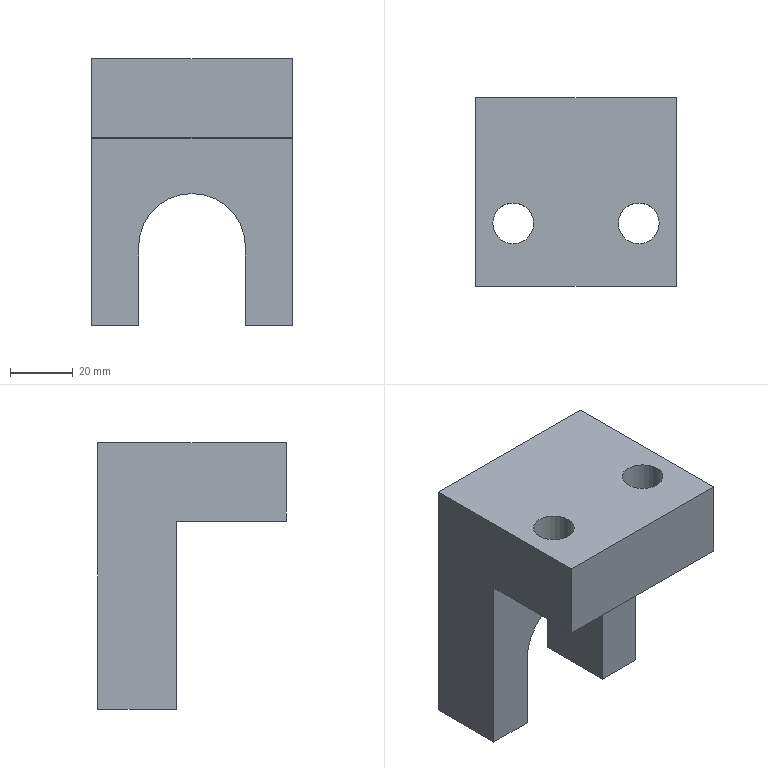Part | NX | features solid 2 | 1 solid | 19 faces | box 64 x 60 x 85 mm | volume 147325 mm3 | plane 13 | cylinder 6 | commonest cylinder face diameters 13 x2 20 x2 1 x1 34 x1
STEP:
#1=CARTESIAN_POINT('',(-138.,919.,-335.));
#2=VERTEX_POINT('',#1);
#3=CARTESIAN_POINT('',(-138.,919.,-310.));
#4=VERTEX_POINT('',#3);
#5=CARTESIAN_POINT('',(-138.,919.,-335.));
#6=DIRECTION('',(0.,0.,1.));
#7=VECTOR('',#6,1000.);
#8=LINE('',#5,#7);
#9=EDGE_CURVE('',#2,#4,#8,.T.);
#10=ORIENTED_EDGE('',*,*,#9,.T.);
#11=CARTESIAN_POINT('',(-202.,919.,-310.));
#12=VERTEX_POINT('',#11);
#13=CARTESIAN_POINT('',(-202.,919.,-310.));
#14=DIRECTION('',(-1.,0.,0.));
#15=VECTOR('',#14,1000.);
#16=LINE('',#13,#15);
#17=EDGE_CURVE('',#4,#12,#16,.T.);
#18=ORIENTED_EDGE('',*,*,#17,.T.);
#19=CARTESIAN_POINT('',(-202.,919.,-335.));
#20=VERTEX_POINT('',#19);
#21=CARTESIAN_POINT('',(-202.,919.,-335.));
#22=DIRECTION('',(0.,0.,-1.));
#23=VECTOR('',#22,1000.);
#24=LINE('',#21,#23);
#25=EDGE_CURVE('',#12,#20,#24,.T.);
#26=ORIENTED_EDGE('',*,*,#25,.T.);
#27=CARTESIAN_POINT('',(-202.,919.,-335.));
#28=DIRECTION('',(1.,0.,0.));
#29=VECTOR('',#28,1000.);
#30=LINE('',#27,#29);
#31=EDGE_CURVE('',#20,#2,#30,.T.);
#32=ORIENTED_EDGE('',*,*,#31,.T.);
#33=EDGE_LOOP('',(#10,#18,#26,#32));
#34=FACE_BOUND('',#33,.T.);
#35=CARTESIAN_POINT('',(-202.,919.,-335.));
#36=DIRECTION('',(0.,1.,0.));
#37=DIRECTION('',(-1.,0.,0.));
#38=AXIS2_PLACEMENT_3D('',#35,#36,#37);
#39=PLANE('',#38);
#40=ADVANCED_FACE('',(#34),#39,.F.);
#41=CARTESIAN_POINT('',(-153.,979.,-395.));
#42=VERTEX_POINT('',#41);
#43=CARTESIAN_POINT('',(-153.,954.,-395.));
#44=VERTEX_POINT('',#43);
#45=CARTESIAN_POINT('',(-153.,979.,-395.));
#46=DIRECTION('',(0.,-1.,0.));
#47=VECTOR('',#46,1000.);
#48=LINE('',#45,#47);
#49=EDGE_CURVE('',#42,#44,#48,.T.);
#50=ORIENTED_EDGE('',*,*,#49,.F.);
#51=CARTESIAN_POINT('',(-138.,979.,-395.));
#52=VERTEX_POINT('',#51);
#53=CARTESIAN_POINT('',(-138.,979.,-395.));
#54=DIRECTION('',(1.,0.,0.));
#55=VECTOR('',#54,1000.);
#56=LINE('',#53,#55);
#57=EDGE_CURVE('',#42,#52,#56,.T.);
#58=ORIENTED_EDGE('',*,*,#57,.T.);
#59=CARTESIAN_POINT('',(-138.,954.,-395.));
#60=VERTEX_POINT('',#59);
#61=CARTESIAN_POINT('',(-138.,979.,-395.));
#62=DIRECTION('',(0.,-1.,0.));
#63=VECTOR('',#62,1000.);
#64=LINE('',#61,#63);
#65=EDGE_CURVE('',#52,#60,#64,.T.);
#66=ORIENTED_EDGE('',*,*,#65,.T.);
#67=CARTESIAN_POINT('',(-138.,954.,-395.));
#68=DIRECTION('',(1.,0.,0.));
#69=VECTOR('',#68,1000.);
#70=LINE('',#67,#69);
#71=EDGE_CURVE('',#44,#60,#70,.T.);
#72=ORIENTED_EDGE('',*,*,#71,.F.);
#73=EDGE_LOOP('',(#50,#58,#66,#72));
#74=FACE_BOUND('',#73,.T.);
#75=CARTESIAN_POINT('',(-138.,979.,-395.));
#76=DIRECTION('',(0.,0.,1.));
#77=DIRECTION('',(0.,1.,0.));
#78=AXIS2_PLACEMENT_3D('',#75,#76,#77);
#79=PLANE('',#78);
#80=ADVANCED_FACE('',(#74),#79,.F.);
#81=CARTESIAN_POINT('',(-187.,954.,-395.));
#82=VERTEX_POINT('',#81);
#83=CARTESIAN_POINT('',(-187.,979.,-395.));
#84=VERTEX_POINT('',#83);
#85=CARTESIAN_POINT('',(-187.,979.,-395.));
#86=DIRECTION('',(0.,1.,0.));
#87=VECTOR('',#86,1000.);
#88=LINE('',#85,#87);
#89=EDGE_CURVE('',#82,#84,#88,.T.);
#90=ORIENTED_EDGE('',*,*,#89,.F.);
#91=CARTESIAN_POINT('',(-202.,954.,-395.));
#92=VERTEX_POINT('',#91);
#93=CARTESIAN_POINT('',(-138.,954.,-395.));
#94=DIRECTION('',(1.,0.,0.));
#95=VECTOR('',#94,1000.);
#96=LINE('',#93,#95);
#97=EDGE_CURVE('',#92,#82,#96,.T.);
#98=ORIENTED_EDGE('',*,*,#97,.F.);
#99=CARTESIAN_POINT('',(-202.,979.,-395.));
#100=VERTEX_POINT('',#99);
#101=CARTESIAN_POINT('',(-202.,979.,-395.));
#102=DIRECTION('',(0.,1.,0.));
#103=VECTOR('',#102,1000.);
#104=LINE('',#101,#103);
#105=EDGE_CURVE('',#92,#100,#104,.T.);
#106=ORIENTED_EDGE('',*,*,#105,.T.);
#107=CARTESIAN_POINT('',(-138.,979.,-395.));
#108=DIRECTION('',(1.,0.,0.));
#109=VECTOR('',#108,1000.);
#110=LINE('',#107,#109);
#111=EDGE_CURVE('',#100,#84,#110,.T.);
#112=ORIENTED_EDGE('',*,*,#111,.T.);
#113=EDGE_LOOP('',(#90,#98,#106,#112));
#114=FACE_BOUND('',#113,.T.);
#115=CARTESIAN_POINT('',(-138.,979.,-395.));
#116=DIRECTION('',(0.,0.,1.));
#117=DIRECTION('',(0.,1.,0.));
#118=AXIS2_PLACEMENT_3D('',#115,#116,#117);
#119=PLANE('',#118);
#120=ADVANCED_FACE('',(#114),#119,.F.);
#121=CARTESIAN_POINT('',(-138.,979.,-310.));
#122=VERTEX_POINT('',#121);
#123=CARTESIAN_POINT('',(-202.,979.,-310.));
#124=VERTEX_POINT('',#123);
#125=CARTESIAN_POINT('',(-202.,979.,-310.));
#126=DIRECTION('',(-1.,0.,0.));
#127=VECTOR('',#126,1000.);
#128=LINE('',#125,#127);
#129=EDGE_CURVE('',#122,#124,#128,.T.);
#130=ORIENTED_EDGE('',*,*,#129,.F.);
#131=CARTESIAN_POINT('',(-138.,979.,-335.));
#132=DIRECTION('',(0.,0.,-1.));
#133=VECTOR('',#132,1000.);
#134=LINE('',#131,#133);
#135=EDGE_CURVE('',#122,#52,#134,.T.);
#136=ORIENTED_EDGE('',*,*,#135,.T.);
#137=ORIENTED_EDGE('',*,*,#57,.F.);
#138=CARTESIAN_POINT('',(-153.,979.,-370.));
#139=VERTEX_POINT('',#138);
#140=CARTESIAN_POINT('',(-153.,979.,-370.));
#141=DIRECTION('',(0.,0.,-1.));
#142=VECTOR('',#141,1000.);
#143=LINE('',#140,#142);
#144=EDGE_CURVE('',#139,#42,#143,.T.);
#145=ORIENTED_EDGE('',*,*,#144,.F.);
#146=CARTESIAN_POINT('',(-187.,979.,-370.));
#147=VERTEX_POINT('',#146);
#148=CARTESIAN_POINT('',(-170.,979.,-370.));
#149=DIRECTION('',(0.,1.,0.));
#150=DIRECTION('',(-1.,0.,0.));
#151=AXIS2_PLACEMENT_3D('',#148,#149,#150);
#152=CIRCLE('',#151,17.);
#153=EDGE_CURVE('',#147,#139,#152,.T.);
#154=ORIENTED_EDGE('',*,*,#153,.F.);
#155=CARTESIAN_POINT('',(-187.,979.,-390.));
#156=DIRECTION('',(0.,0.,1.));
#157=VECTOR('',#156,1000.);
#158=LINE('',#155,#157);
#159=EDGE_CURVE('',#84,#147,#158,.T.);
#160=ORIENTED_EDGE('',*,*,#159,.F.);
#161=ORIENTED_EDGE('',*,*,#111,.F.);
#162=CARTESIAN_POINT('',(-202.,979.,-335.));
#163=DIRECTION('',(0.,0.,1.));
#164=VECTOR('',#163,1000.);
#165=LINE('',#162,#164);
#166=EDGE_CURVE('',#100,#124,#165,.T.);
#167=ORIENTED_EDGE('',*,*,#166,.T.);
#168=EDGE_LOOP('',(#130,#136,#137,#145,#154,#160,#161,#167));
#169=FACE_BOUND('',#168,.T.);
#170=CARTESIAN_POINT('',(-138.,979.,-310.));
#171=DIRECTION('',(0.,-1.,0.));
#172=DIRECTION('',(1.,0.,0.));
#173=AXIS2_PLACEMENT_3D('',#170,#171,#172);
#174=PLANE('',#173);
#175=ADVANCED_FACE('',(#169),#174,.F.);
#176=CARTESIAN_POINT('',(-153.,954.,-370.));
#177=VERTEX_POINT('',#176);
#178=CARTESIAN_POINT('',(-153.,954.,-370.));
#179=DIRECTION('',(0.,0.,-1.));
#180=VECTOR('',#179,1000.);
#181=LINE('',#178,#180);
#182=EDGE_CURVE('',#177,#44,#181,.T.);
#183=ORIENTED_EDGE('',*,*,#182,.T.);
#184=ORIENTED_EDGE('',*,*,#71,.T.);
#185=CARTESIAN_POINT('',(-138.,954.,-335.5));
#186=VERTEX_POINT('',#185);
#187=CARTESIAN_POINT('',(-138.,954.,-335.));
#188=DIRECTION('',(0.,0.,-1.));
#189=VECTOR('',#188,1000.);
#190=LINE('',#187,#189);
#191=EDGE_CURVE('',#186,#60,#190,.T.);
#192=ORIENTED_EDGE('',*,*,#191,.F.);
#193=CARTESIAN_POINT('',(-202.,954.,-335.5));
#194=VERTEX_POINT('',#193);
#195=CARTESIAN_POINT('',(-138.,954.,-335.5));
#196=DIRECTION('',(1.,0.,0.));
#197=VECTOR('',#196,1000.);
#198=LINE('',#195,#197);
#199=EDGE_CURVE('',#186,#194,#198,.F.);
#200=ORIENTED_EDGE('',*,*,#199,.T.);
#201=CARTESIAN_POINT('',(-202.,954.,-335.));
#202=DIRECTION('',(0.,0.,1.));
#203=VECTOR('',#202,1000.);
#204=LINE('',#201,#203);
#205=EDGE_CURVE('',#92,#194,#204,.T.);
#206=ORIENTED_EDGE('',*,*,#205,.F.);
#207=ORIENTED_EDGE('',*,*,#97,.T.);
#208=CARTESIAN_POINT('',(-187.,954.,-370.));
#209=VERTEX_POINT('',#208);
#210=CARTESIAN_POINT('',(-187.,954.,-390.));
#211=DIRECTION('',(0.,0.,1.));
#212=VECTOR('',#211,1000.);
#213=LINE('',#210,#212);
#214=EDGE_CURVE('',#82,#209,#213,.T.);
#215=ORIENTED_EDGE('',*,*,#214,.T.);
#216=CARTESIAN_POINT('',(-170.,954.,-370.));
#217=DIRECTION('',(0.,1.,0.));
#218=DIRECTION('',(-1.,0.,0.));
#219=AXIS2_PLACEMENT_3D('',#216,#217,#218);
#220=CIRCLE('',#219,17.);
#221=EDGE_CURVE('',#209,#177,#220,.T.);
#222=ORIENTED_EDGE('',*,*,#221,.T.);
#223=EDGE_LOOP('',(#183,#184,#192,#200,#206,#207,#215,#222));
#224=FACE_BOUND('',#223,.T.);
#225=CARTESIAN_POINT('',(-138.,954.,-310.));
#226=DIRECTION('',(0.,-1.,0.));
#227=DIRECTION('',(1.,0.,0.));
#228=AXIS2_PLACEMENT_3D('',#225,#226,#227);
#229=PLANE('',#228);
#230=ADVANCED_FACE('',(#224),#229,.T.);
#231=ORIENTED_EDGE('',*,*,#9,.F.);
#232=CARTESIAN_POINT('',(-138.,953.5,-335.));
#233=VERTEX_POINT('',#232);
#234=CARTESIAN_POINT('',(-138.,919.,-335.));
#235=DIRECTION('',(0.,1.,0.));
#236=VECTOR('',#235,1000.);
#237=LINE('',#234,#236);
#238=EDGE_CURVE('',#2,#233,#237,.T.);
#239=ORIENTED_EDGE('',*,*,#238,.T.);
#240=CARTESIAN_POINT('',(-138.,953.5,-335.5));
#241=DIRECTION('',(-1.,0.,0.));
#242=DIRECTION('',(0.,-1.,0.));
#243=AXIS2_PLACEMENT_3D('',#240,#241,#242);
#244=CIRCLE('',#243,0.5);
#245=EDGE_CURVE('',#233,#186,#244,.T.);
#246=ORIENTED_EDGE('',*,*,#245,.T.);
#247=ORIENTED_EDGE('',*,*,#191,.T.);
#248=ORIENTED_EDGE('',*,*,#65,.F.);
#249=ORIENTED_EDGE('',*,*,#135,.F.);
#250=CARTESIAN_POINT('',(-138.,979.,-310.));
#251=DIRECTION('',(0.,-1.,0.));
#252=VECTOR('',#251,1000.);
#253=LINE('',#250,#252);
#254=EDGE_CURVE('',#122,#4,#253,.T.);
#255=ORIENTED_EDGE('',*,*,#254,.T.);
#256=EDGE_LOOP('',(#231,#239,#246,#247,#248,#249,#255));
#257=FACE_BOUND('',#256,.T.);
#258=CARTESIAN_POINT('',(-138.,979.,-335.));
#259=DIRECTION('',(-1.,0.,0.));
#260=DIRECTION('',(0.,-1.,0.));
#261=AXIS2_PLACEMENT_3D('',#258,#259,#260);
#262=PLANE('',#261);
#263=ADVANCED_FACE('',(#257),#262,.F.);
#264=ORIENTED_EDGE('',*,*,#25,.F.);
#265=CARTESIAN_POINT('',(-202.,979.,-310.));
#266=DIRECTION('',(0.,-1.,0.));
#267=VECTOR('',#266,1000.);
#268=LINE('',#265,#267);
#269=EDGE_CURVE('',#124,#12,#268,.T.);
#270=ORIENTED_EDGE('',*,*,#269,.F.);
#271=ORIENTED_EDGE('',*,*,#166,.F.);
#272=ORIENTED_EDGE('',*,*,#105,.F.);
#273=ORIENTED_EDGE('',*,*,#205,.T.);
#274=CARTESIAN_POINT('',(-202.,953.5,-335.));
#275=VERTEX_POINT('',#274);
#276=CARTESIAN_POINT('',(-202.,953.5,-335.5));
#277=DIRECTION('',(1.,0.,0.));
#278=DIRECTION('',(0.,1.,0.));
#279=AXIS2_PLACEMENT_3D('',#276,#277,#278);
#280=CIRCLE('',#279,0.5);
#281=EDGE_CURVE('',#194,#275,#280,.T.);
#282=ORIENTED_EDGE('',*,*,#281,.T.);
#283=CARTESIAN_POINT('',(-202.,919.,-335.));
#284=DIRECTION('',(0.,1.,0.));
#285=VECTOR('',#284,1000.);
#286=LINE('',#283,#285);
#287=EDGE_CURVE('',#20,#275,#286,.T.);
#288=ORIENTED_EDGE('',*,*,#287,.F.);
#289=EDGE_LOOP('',(#264,#270,#271,#272,#273,#282,#288));
#290=FACE_BOUND('',#289,.T.);
#291=CARTESIAN_POINT('',(-202.,979.,-335.));
#292=DIRECTION('',(1.,0.,0.));
#293=DIRECTION('',(0.,1.,0.));
#294=AXIS2_PLACEMENT_3D('',#291,#292,#293);
#295=PLANE('',#294);
#296=ADVANCED_FACE('',(#290),#295,.F.);
#297=ORIENTED_EDGE('',*,*,#17,.F.);
#298=ORIENTED_EDGE('',*,*,#254,.F.);
#299=ORIENTED_EDGE('',*,*,#129,.T.);
#300=ORIENTED_EDGE('',*,*,#269,.T.);
#301=EDGE_LOOP('',(#297,#298,#299,#300));
#302=FACE_BOUND('',#301,.T.);
#303=CARTESIAN_POINT('',(-156.5,939.,-310.));
#304=VERTEX_POINT('',#303);
#305=CARTESIAN_POINT('',(-150.,939.,-310.));
#306=DIRECTION('',(0.,0.,-1.));
#307=DIRECTION('',(-1.,0.,0.));
#308=AXIS2_PLACEMENT_3D('',#305,#306,#307);
#309=CIRCLE('',#308,6.5);
#310=EDGE_CURVE('',#304,#304,#309,.T.);
#311=ORIENTED_EDGE('',*,*,#310,.T.);
#312=EDGE_LOOP('',(#311));
#313=FACE_BOUND('',#312,.T.);
#314=CARTESIAN_POINT('',(-196.5,939.,-310.));
#315=VERTEX_POINT('',#314);
#316=CARTESIAN_POINT('',(-190.,939.,-310.));
#317=DIRECTION('',(0.,0.,-1.));
#318=DIRECTION('',(-1.,0.,0.));
#319=AXIS2_PLACEMENT_3D('',#316,#317,#318);
#320=CIRCLE('',#319,6.5);
#321=EDGE_CURVE('',#315,#315,#320,.T.);
#322=ORIENTED_EDGE('',*,*,#321,.T.);
#323=EDGE_LOOP('',(#322));
#324=FACE_BOUND('',#323,.T.);
#325=CARTESIAN_POINT('',(-202.,979.,-310.));
#326=DIRECTION('',(0.,0.,-1.));
#327=DIRECTION('',(-1.,0.,0.));
#328=AXIS2_PLACEMENT_3D('',#325,#326,#327);
#329=PLANE('',#328);
#330=ADVANCED_FACE('',(#302,#313,#324),#329,.F.);
#331=ORIENTED_EDGE('',*,*,#31,.F.);
#332=ORIENTED_EDGE('',*,*,#287,.T.);
#333=CARTESIAN_POINT('',(-202.,953.5,-335.));
#334=DIRECTION('',(1.,0.,0.));
#335=VECTOR('',#334,1000.);
#336=LINE('',#333,#335);
#337=EDGE_CURVE('',#275,#233,#336,.T.);
#338=ORIENTED_EDGE('',*,*,#337,.T.);
#339=ORIENTED_EDGE('',*,*,#238,.F.);
#340=EDGE_LOOP('',(#331,#332,#338,#339));
#341=FACE_BOUND('',#340,.T.);
#342=CARTESIAN_POINT('',(-140.,939.,-335.));
#343=VERTEX_POINT('',#342);
#344=CARTESIAN_POINT('',(-150.,939.,-335.));
#345=DIRECTION('',(0.,0.,1.));
#346=DIRECTION('',(1.,0.,0.));
#347=AXIS2_PLACEMENT_3D('',#344,#345,#346);
#348=CIRCLE('',#347,10.);
#349=EDGE_CURVE('',#343,#343,#348,.T.);
#350=ORIENTED_EDGE('',*,*,#349,.T.);
#351=EDGE_LOOP('',(#350));
#352=FACE_BOUND('',#351,.T.);
#353=CARTESIAN_POINT('',(-180.,939.,-335.));
#354=VERTEX_POINT('',#353);
#355=CARTESIAN_POINT('',(-190.,939.,-335.));
#356=DIRECTION('',(0.,0.,1.));
#357=DIRECTION('',(1.,0.,0.));
#358=AXIS2_PLACEMENT_3D('',#355,#356,#357);
#359=CIRCLE('',#358,10.);
#360=EDGE_CURVE('',#354,#354,#359,.T.);
#361=ORIENTED_EDGE('',*,*,#360,.T.);
#362=EDGE_LOOP('',(#361));
#363=FACE_BOUND('',#362,.T.);
#364=CARTESIAN_POINT('',(-202.,919.,-335.));
#365=DIRECTION('',(0.,0.,1.));
#366=DIRECTION('',(0.,1.,0.));
#367=AXIS2_PLACEMENT_3D('',#364,#365,#366);
#368=PLANE('',#367);
#369=ADVANCED_FACE('',(#341,#352,#363),#368,.F.);
#370=ORIENTED_EDGE('',*,*,#214,.F.);
#371=ORIENTED_EDGE('',*,*,#89,.T.);
#372=ORIENTED_EDGE('',*,*,#159,.T.);
#373=CARTESIAN_POINT('',(-187.,979.,-370.));
#374=DIRECTION('',(0.,-1.,0.));
#375=VECTOR('',#374,1000.);
#376=LINE('',#373,#375);
#377=EDGE_CURVE('',#147,#209,#376,.T.);
#378=ORIENTED_EDGE('',*,*,#377,.T.);
#379=EDGE_LOOP('',(#370,#371,#372,#378));
#380=FACE_BOUND('',#379,.T.);
#381=CARTESIAN_POINT('',(-187.,979.,-390.));
#382=DIRECTION('',(1.,0.,0.));
#383=DIRECTION('',(0.,0.,-1.));
#384=AXIS2_PLACEMENT_3D('',#381,#382,#383);
#385=PLANE('',#384);
#386=ADVANCED_FACE('',(#380),#385,.T.);
#387=ORIENTED_EDGE('',*,*,#221,.F.);
#388=ORIENTED_EDGE('',*,*,#377,.F.);
#389=ORIENTED_EDGE('',*,*,#153,.T.);
#390=CARTESIAN_POINT('',(-153.,979.,-370.));
#391=DIRECTION('',(0.,-1.,0.));
#392=VECTOR('',#391,1000.);
#393=LINE('',#390,#392);
#394=EDGE_CURVE('',#139,#177,#393,.T.);
#395=ORIENTED_EDGE('',*,*,#394,.T.);
#396=EDGE_LOOP('',(#387,#388,#389,#395));
#397=FACE_BOUND('',#396,.T.);
#398=CARTESIAN_POINT('',(-170.,979.,-370.));
#399=DIRECTION('',(0.,-1.,0.));
#400=DIRECTION('',(1.,0.,0.));
#401=AXIS2_PLACEMENT_3D('',#398,#399,#400);
#402=CYLINDRICAL_SURFACE('',#401,17.);
#403=ADVANCED_FACE('',(#397),#402,.F.);
#404=ORIENTED_EDGE('',*,*,#144,.T.);
#405=ORIENTED_EDGE('',*,*,#49,.T.);
#406=ORIENTED_EDGE('',*,*,#182,.F.);
#407=ORIENTED_EDGE('',*,*,#394,.F.);
#408=EDGE_LOOP('',(#404,#405,#406,#407));
#409=FACE_BOUND('',#408,.T.);
#410=CARTESIAN_POINT('',(-153.,979.,-370.));
#411=DIRECTION('',(-1.,0.,0.));
#412=DIRECTION('',(0.,0.,1.));
#413=AXIS2_PLACEMENT_3D('',#410,#411,#412);
#414=PLANE('',#413);
#415=ADVANCED_FACE('',(#409),#414,.T.);
#416=CARTESIAN_POINT('',(-183.5,939.,-320.));
#417=VERTEX_POINT('',#416);
#418=CARTESIAN_POINT('',(-190.,939.,-320.));
#419=DIRECTION('',(0.,0.,1.));
#420=DIRECTION('',(1.,0.,0.));
#421=AXIS2_PLACEMENT_3D('',#418,#419,#420);
#422=CIRCLE('',#421,6.5);
#423=EDGE_CURVE('',#417,#417,#422,.T.);
#424=ORIENTED_EDGE('',*,*,#423,.F.);
#425=EDGE_LOOP('',(#424));
#426=FACE_BOUND('',#425,.T.);
#427=ORIENTED_EDGE('',*,*,#321,.F.);
#428=EDGE_LOOP('',(#427));
#429=FACE_BOUND('',#428,.T.);
#430=CARTESIAN_POINT('',(-190.,939.,-285.));
#431=DIRECTION('',(0.,0.,1.));
#432=DIRECTION('',(0.,1.,0.));
#433=AXIS2_PLACEMENT_3D('',#430,#431,#432);
#434=CYLINDRICAL_SURFACE('',#433,6.5);
#435=ADVANCED_FACE('',(#426,#429),#434,.F.);
#436=ORIENTED_EDGE('',*,*,#423,.T.);
#437=EDGE_LOOP('',(#436));
#438=FACE_BOUND('',#437,.T.);
#439=CARTESIAN_POINT('',(-180.,939.,-320.));
#440=VERTEX_POINT('',#439);
#441=CARTESIAN_POINT('',(-190.,939.,-320.));
#442=DIRECTION('',(0.,0.,1.));
#443=DIRECTION('',(1.,0.,0.));
#444=AXIS2_PLACEMENT_3D('',#441,#442,#443);
#445=CIRCLE('',#444,10.);
#446=EDGE_CURVE('',#440,#440,#445,.T.);
#447=ORIENTED_EDGE('',*,*,#446,.F.);
#448=EDGE_LOOP('',(#447));
#449=FACE_BOUND('',#448,.T.);
#450=CARTESIAN_POINT('',(-190.,939.,-320.));
#451=DIRECTION('',(0.,0.,1.));
#452=DIRECTION('',(0.,1.,0.));
#453=AXIS2_PLACEMENT_3D('',#450,#451,#452);
#454=PLANE('',#453);
#455=ADVANCED_FACE('',(#438,#449),#454,.F.);
#456=ORIENTED_EDGE('',*,*,#446,.T.);
#457=EDGE_LOOP('',(#456));
#458=FACE_BOUND('',#457,.T.);
#459=ORIENTED_EDGE('',*,*,#360,.F.);
#460=EDGE_LOOP('',(#459));
#461=FACE_BOUND('',#460,.T.);
#462=CARTESIAN_POINT('',(-190.,939.,-335.));
#463=DIRECTION('',(0.,0.,1.));
#464=DIRECTION('',(0.,1.,0.));
#465=AXIS2_PLACEMENT_3D('',#462,#463,#464);
#466=CYLINDRICAL_SURFACE('',#465,10.);
#467=ADVANCED_FACE('',(#458,#461),#466,.F.);
#468=CARTESIAN_POINT('',(-143.5,939.,-320.));
#469=VERTEX_POINT('',#468);
#470=CARTESIAN_POINT('',(-150.,939.,-320.));
#471=DIRECTION('',(0.,0.,1.));
#472=DIRECTION('',(1.,0.,0.));
#473=AXIS2_PLACEMENT_3D('',#470,#471,#472);
#474=CIRCLE('',#473,6.5);
#475=EDGE_CURVE('',#469,#469,#474,.T.);
#476=ORIENTED_EDGE('',*,*,#475,.F.);
#477=EDGE_LOOP('',(#476));
#478=FACE_BOUND('',#477,.T.);
#479=ORIENTED_EDGE('',*,*,#310,.F.);
#480=EDGE_LOOP('',(#479));
#481=FACE_BOUND('',#480,.T.);
#482=CARTESIAN_POINT('',(-150.,939.,-285.));
#483=DIRECTION('',(0.,0.,1.));
#484=DIRECTION('',(0.,1.,0.));
#485=AXIS2_PLACEMENT_3D('',#482,#483,#484);
#486=CYLINDRICAL_SURFACE('',#485,6.5);
#487=ADVANCED_FACE('',(#478,#481),#486,.F.);
#488=ORIENTED_EDGE('',*,*,#475,.T.);
#489=EDGE_LOOP('',(#488));
#490=FACE_BOUND('',#489,.T.);
#491=CARTESIAN_POINT('',(-140.,939.,-320.));
#492=VERTEX_POINT('',#491);
#493=CARTESIAN_POINT('',(-150.,939.,-320.));
#494=DIRECTION('',(0.,0.,1.));
#495=DIRECTION('',(1.,0.,0.));
#496=AXIS2_PLACEMENT_3D('',#493,#494,#495);
#497=CIRCLE('',#496,10.);
#498=EDGE_CURVE('',#492,#492,#497,.T.);
#499=ORIENTED_EDGE('',*,*,#498,.F.);
#500=EDGE_LOOP('',(#499));
#501=FACE_BOUND('',#500,.T.);
#502=CARTESIAN_POINT('',(-150.,939.,-320.));
#503=DIRECTION('',(0.,0.,1.));
#504=DIRECTION('',(0.,1.,0.));
#505=AXIS2_PLACEMENT_3D('',#502,#503,#504);
#506=PLANE('',#505);
#507=ADVANCED_FACE('',(#490,#501),#506,.F.);
#508=ORIENTED_EDGE('',*,*,#498,.T.);
#509=EDGE_LOOP('',(#508));
#510=FACE_BOUND('',#509,.T.);
#511=ORIENTED_EDGE('',*,*,#349,.F.);
#512=EDGE_LOOP('',(#511));
#513=FACE_BOUND('',#512,.T.);
#514=CARTESIAN_POINT('',(-150.,939.,-335.));
#515=DIRECTION('',(0.,0.,1.));
#516=DIRECTION('',(0.,1.,0.));
#517=AXIS2_PLACEMENT_3D('',#514,#515,#516);
#518=CYLINDRICAL_SURFACE('',#517,10.);
#519=ADVANCED_FACE('',(#510,#513),#518,.F.);
#520=ORIENTED_EDGE('',*,*,#281,.F.);
#521=ORIENTED_EDGE('',*,*,#199,.F.);
#522=ORIENTED_EDGE('',*,*,#245,.F.);
#523=ORIENTED_EDGE('',*,*,#337,.F.);
#524=EDGE_LOOP('',(#520,#521,#522,#523));
#525=FACE_BOUND('',#524,.T.);
#526=CARTESIAN_POINT('',(-202.,953.5,-335.5));
#527=DIRECTION('',(1.,0.,0.));
#528=DIRECTION('',(0.,1.,0.));
#529=AXIS2_PLACEMENT_3D('',#526,#527,#528);
#530=CYLINDRICAL_SURFACE('',#529,0.5);
#531=ADVANCED_FACE('',(#525),#530,.F.);
#532=CLOSED_SHELL('',(#40,#80,#120,#175,#230,#263,#296,#330,#369,#386,#403,#415,#435,#455,#467,#487,#507,#519,#531));
#533=MANIFOLD_SOLID_BREP('',#532);
#534=(LENGTH_UNIT()NAMED_UNIT(*)SI_UNIT(.MILLI.,.METRE.));
#535=UNCERTAINTY_MEASURE_WITH_UNIT(LENGTH_MEASURE(0.00001),#534,'','');
#536=(NAMED_UNIT(*)PLANE_ANGLE_UNIT()SI_UNIT($,.RADIAN.));
#537=(NAMED_UNIT(*)SI_UNIT($,.STERADIAN.)SOLID_ANGLE_UNIT());
#538=(GEOMETRIC_REPRESENTATION_CONTEXT(3)GLOBAL_UNCERTAINTY_ASSIGNED_CONTEXT((#535))GLOBAL_UNIT_ASSIGNED_CONTEXT((#534,#536,#537))REPRESENTATION_CONTEXT('',''));
#539=ADVANCED_BREP_SHAPE_REPRESENTATION('',(#533),#538);